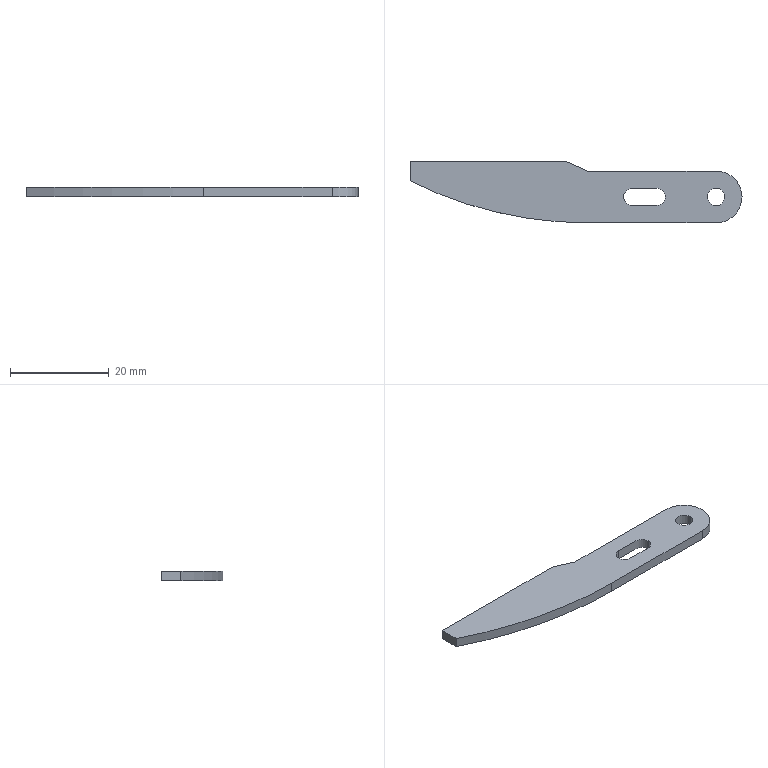Part | SolidWorks | features SMBaseFlange 2, FlatPattern 1, ICE 1, SheetMetal 1 | 1 solid | 17 faces | box 67.25 x 12.5 x 2 mm | volume 1251 mm3 | plane 9 | cylinder 8 | commonest cylinder face diameters 3.5 x5 10.5 x2 160.971 x1
STEP:
#1=CARTESIAN_POINT('',(2.75,0.,-2.));
#2=VERTEX_POINT('',#1);
#3=CARTESIAN_POINT('',(1.,1.75,-2.));
#4=VERTEX_POINT('',#3);
#5=CARTESIAN_POINT('',(1.,0.,-2.));
#6=DIRECTION('',(0.,0.,1.));
#7=DIRECTION('',(1.,0.,0.));
#8=AXIS2_PLACEMENT_3D('',#5,#6,#7);
#9=CIRCLE('',#8,1.75);
#10=EDGE_CURVE('',#2,#4,#9,.T.);
#11=ORIENTED_EDGE('',*,*,#10,.F.);
#12=CARTESIAN_POINT('',(2.75,0.,0.));
#13=VERTEX_POINT('',#12);
#14=CARTESIAN_POINT('',(2.75,0.,-2.));
#15=DIRECTION('',(0.,0.,1.));
#16=VECTOR('',#15,1000.);
#17=LINE('',#14,#16);
#18=EDGE_CURVE('',#2,#13,#17,.T.);
#19=ORIENTED_EDGE('',*,*,#18,.T.);
#20=CARTESIAN_POINT('',(1.,1.75,0.));
#21=VERTEX_POINT('',#20);
#22=CARTESIAN_POINT('',(1.,0.,0.));
#23=DIRECTION('',(0.,0.,1.));
#24=DIRECTION('',(1.,0.,0.));
#25=AXIS2_PLACEMENT_3D('',#22,#23,#24);
#26=CIRCLE('',#25,1.75);
#27=EDGE_CURVE('',#13,#21,#26,.T.);
#28=ORIENTED_EDGE('',*,*,#27,.T.);
#29=CARTESIAN_POINT('',(1.,1.75,-2.));
#30=DIRECTION('',(0.,0.,1.));
#31=VECTOR('',#30,1000.);
#32=LINE('',#29,#31);
#33=EDGE_CURVE('',#4,#21,#32,.T.);
#34=ORIENTED_EDGE('',*,*,#33,.F.);
#35=EDGE_LOOP('',(#11,#19,#28,#34));
#36=FACE_OUTER_BOUND('',#35,.T.);
#37=CARTESIAN_POINT('',(1.,0.,-2.));
#38=DIRECTION('',(0.,0.,1.));
#39=DIRECTION('',(1.,0.,0.));
#40=AXIS2_PLACEMENT_3D('',#37,#38,#39);
#41=CYLINDRICAL_SURFACE('',#40,1.75);
#42=ADVANCED_FACE('',(#36),#41,.F.);
#43=CARTESIAN_POINT('',(11.25,0.,-2.));
#44=VERTEX_POINT('',#43);
#45=CARTESIAN_POINT('',(14.75,0.,-2.));
#46=VERTEX_POINT('',#45);
#47=CARTESIAN_POINT('',(13.,0.,-2.));
#48=DIRECTION('',(0.,0.,1.));
#49=DIRECTION('',(1.,0.,0.));
#50=AXIS2_PLACEMENT_3D('',#47,#48,#49);
#51=CIRCLE('',#50,1.75);
#52=EDGE_CURVE('',#44,#46,#51,.T.);
#53=ORIENTED_EDGE('',*,*,#52,.F.);
#54=CARTESIAN_POINT('',(11.25,0.,0.));
#55=VERTEX_POINT('',#54);
#56=CARTESIAN_POINT('',(11.25,0.,-2.));
#57=DIRECTION('',(0.,0.,1.));
#58=VECTOR('',#57,1000.);
#59=LINE('',#56,#58);
#60=EDGE_CURVE('',#44,#55,#59,.T.);
#61=ORIENTED_EDGE('',*,*,#60,.T.);
#62=CARTESIAN_POINT('',(14.75,0.,0.));
#63=VERTEX_POINT('',#62);
#64=CARTESIAN_POINT('',(13.,0.,0.));
#65=DIRECTION('',(0.,0.,1.));
#66=DIRECTION('',(1.,0.,0.));
#67=AXIS2_PLACEMENT_3D('',#64,#65,#66);
#68=CIRCLE('',#67,1.75);
#69=EDGE_CURVE('',#55,#63,#68,.T.);
#70=ORIENTED_EDGE('',*,*,#69,.T.);
#71=CARTESIAN_POINT('',(14.75,0.,-2.));
#72=DIRECTION('',(0.,0.,1.));
#73=VECTOR('',#72,1000.);
#74=LINE('',#71,#73);
#75=EDGE_CURVE('',#46,#63,#74,.T.);
#76=ORIENTED_EDGE('',*,*,#75,.F.);
#77=EDGE_LOOP('',(#53,#61,#70,#76));
#78=FACE_OUTER_BOUND('',#77,.T.);
#79=CARTESIAN_POINT('',(13.,0.,-2.));
#80=DIRECTION('',(0.,0.,1.));
#81=DIRECTION('',(1.,0.,0.));
#82=AXIS2_PLACEMENT_3D('',#79,#80,#81);
#83=CYLINDRICAL_SURFACE('',#82,1.75);
#84=ADVANCED_FACE('',(#78),#83,.F.);
#85=CARTESIAN_POINT('',(13.,-5.25,-2.));
#86=VERTEX_POINT('',#85);
#87=CARTESIAN_POINT('',(18.25,0.,-2.));
#88=VERTEX_POINT('',#87);
#89=CARTESIAN_POINT('',(13.,0.,-2.));
#90=DIRECTION('',(0.,0.,1.));
#91=DIRECTION('',(1.,0.,0.));
#92=AXIS2_PLACEMENT_3D('',#89,#90,#91);
#93=CIRCLE('',#92,5.25);
#94=EDGE_CURVE('',#86,#88,#93,.T.);
#95=ORIENTED_EDGE('',*,*,#94,.T.);
#96=CARTESIAN_POINT('',(18.25,0.,0.));
#97=VERTEX_POINT('',#96);
#98=CARTESIAN_POINT('',(18.25,0.,-2.));
#99=DIRECTION('',(0.,0.,1.));
#100=VECTOR('',#99,1000.);
#101=LINE('',#98,#100);
#102=EDGE_CURVE('',#88,#97,#101,.T.);
#103=ORIENTED_EDGE('',*,*,#102,.T.);
#104=CARTESIAN_POINT('',(13.,-5.25,0.));
#105=VERTEX_POINT('',#104);
#106=CARTESIAN_POINT('',(13.,0.,0.));
#107=DIRECTION('',(0.,0.,1.));
#108=DIRECTION('',(1.,0.,0.));
#109=AXIS2_PLACEMENT_3D('',#106,#107,#108);
#110=CIRCLE('',#109,5.25);
#111=EDGE_CURVE('',#105,#97,#110,.T.);
#112=ORIENTED_EDGE('',*,*,#111,.F.);
#113=CARTESIAN_POINT('',(13.,-5.25,-2.));
#114=DIRECTION('',(0.,0.,1.));
#115=VECTOR('',#114,1000.);
#116=LINE('',#113,#115);
#117=EDGE_CURVE('',#86,#105,#116,.T.);
#118=ORIENTED_EDGE('',*,*,#117,.F.);
#119=EDGE_LOOP('',(#95,#103,#112,#118));
#120=FACE_OUTER_BOUND('',#119,.T.);
#121=CARTESIAN_POINT('',(13.,0.,-2.));
#122=DIRECTION('',(0.,0.,1.));
#123=DIRECTION('',(1.,0.,0.));
#124=AXIS2_PLACEMENT_3D('',#121,#122,#123);
#125=CYLINDRICAL_SURFACE('',#124,5.25);
#126=ADVANCED_FACE('',(#120),#125,.T.);
#127=ORIENTED_EDGE('',*,*,#102,.F.);
#128=CARTESIAN_POINT('',(13.,5.25,-2.));
#129=VERTEX_POINT('',#128);
#130=CARTESIAN_POINT('',(13.,0.,-2.));
#131=DIRECTION('',(0.,0.,1.));
#132=DIRECTION('',(1.,0.,0.));
#133=AXIS2_PLACEMENT_3D('',#130,#131,#132);
#134=CIRCLE('',#133,5.25);
#135=EDGE_CURVE('',#88,#129,#134,.T.);
#136=ORIENTED_EDGE('',*,*,#135,.T.);
#137=CARTESIAN_POINT('',(13.,5.25,0.));
#138=VERTEX_POINT('',#137);
#139=CARTESIAN_POINT('',(13.,5.25,-2.));
#140=DIRECTION('',(0.,0.,1.));
#141=VECTOR('',#140,1000.);
#142=LINE('',#139,#141);
#143=EDGE_CURVE('',#129,#138,#142,.T.);
#144=ORIENTED_EDGE('',*,*,#143,.T.);
#145=CARTESIAN_POINT('',(13.,0.,0.));
#146=DIRECTION('',(0.,0.,1.));
#147=DIRECTION('',(1.,0.,0.));
#148=AXIS2_PLACEMENT_3D('',#145,#146,#147);
#149=CIRCLE('',#148,5.25);
#150=EDGE_CURVE('',#97,#138,#149,.T.);
#151=ORIENTED_EDGE('',*,*,#150,.F.);
#152=EDGE_LOOP('',(#127,#136,#144,#151));
#153=FACE_OUTER_BOUND('',#152,.T.);
#154=CARTESIAN_POINT('',(13.,0.,-2.));
#155=DIRECTION('',(0.,0.,1.));
#156=DIRECTION('',(1.,0.,0.));
#157=AXIS2_PLACEMENT_3D('',#154,#155,#156);
#158=CYLINDRICAL_SURFACE('',#157,5.25);
#159=ADVANCED_FACE('',(#153),#158,.T.);
#160=CARTESIAN_POINT('',(-13.,-5.25,0.));
#161=VERTEX_POINT('',#160);
#162=CARTESIAN_POINT('',(-13.,-5.25,0.));
#163=DIRECTION('',(1.,0.,0.));
#164=VECTOR('',#163,1000.);
#165=LINE('',#162,#164);
#166=EDGE_CURVE('',#161,#105,#165,.T.);
#167=ORIENTED_EDGE('',*,*,#166,.F.);
#168=CARTESIAN_POINT('',(-13.,-5.25,-2.));
#169=VERTEX_POINT('',#168);
#170=CARTESIAN_POINT('',(-13.,-5.25,-2.));
#171=DIRECTION('',(0.,0.,1.));
#172=VECTOR('',#171,1000.);
#173=LINE('',#170,#172);
#174=EDGE_CURVE('',#169,#161,#173,.T.);
#175=ORIENTED_EDGE('',*,*,#174,.F.);
#176=CARTESIAN_POINT('',(-13.,-5.25,-2.));
#177=DIRECTION('',(1.,0.,0.));
#178=VECTOR('',#177,1000.);
#179=LINE('',#176,#178);
#180=EDGE_CURVE('',#169,#86,#179,.T.);
#181=ORIENTED_EDGE('',*,*,#180,.T.);
#182=ORIENTED_EDGE('',*,*,#117,.T.);
#183=EDGE_LOOP('',(#167,#175,#181,#182));
#184=FACE_OUTER_BOUND('',#183,.T.);
#185=CARTESIAN_POINT('',(-13.,-5.25,-2.));
#186=DIRECTION('',(0.,-1.,0.));
#187=DIRECTION('',(1.,0.,0.));
#188=AXIS2_PLACEMENT_3D('',#185,#186,#187);
#189=PLANE('',#188);
#190=ADVANCED_FACE('',(#184),#189,.T.);
#191=CARTESIAN_POINT('',(-13.,5.25,0.));
#192=VERTEX_POINT('',#191);
#193=CARTESIAN_POINT('',(-13.,5.25,0.));
#194=DIRECTION('',(-1.,0.,0.));
#195=VECTOR('',#194,1000.);
#196=LINE('',#193,#195);
#197=EDGE_CURVE('',#138,#192,#196,.T.);
#198=ORIENTED_EDGE('',*,*,#197,.F.);
#199=ORIENTED_EDGE('',*,*,#143,.F.);
#200=CARTESIAN_POINT('',(-13.,5.25,-2.));
#201=VERTEX_POINT('',#200);
#202=CARTESIAN_POINT('',(-13.,5.25,-2.));
#203=DIRECTION('',(-1.,0.,0.));
#204=VECTOR('',#203,1000.);
#205=LINE('',#202,#204);
#206=EDGE_CURVE('',#129,#201,#205,.T.);
#207=ORIENTED_EDGE('',*,*,#206,.T.);
#208=CARTESIAN_POINT('',(-13.,5.25,-2.));
#209=DIRECTION('',(0.,0.,1.));
#210=VECTOR('',#209,1000.);
#211=LINE('',#208,#210);
#212=EDGE_CURVE('',#201,#192,#211,.T.);
#213=ORIENTED_EDGE('',*,*,#212,.T.);
#214=EDGE_LOOP('',(#198,#199,#207,#213));
#215=FACE_OUTER_BOUND('',#214,.T.);
#216=CARTESIAN_POINT('',(-13.,5.25,-2.));
#217=DIRECTION('',(0.,1.,0.));
#218=DIRECTION('',(-1.,0.,0.));
#219=AXIS2_PLACEMENT_3D('',#216,#217,#218);
#220=PLANE('',#219);
#221=ADVANCED_FACE('',(#215),#220,.T.);
#222=CARTESIAN_POINT('',(-4.,1.75,-2.));
#223=VERTEX_POINT('',#222);
#224=CARTESIAN_POINT('',(-4.,1.75,-2.));
#225=DIRECTION('',(-1.,0.,0.));
#226=VECTOR('',#225,1000.);
#227=LINE('',#224,#226);
#228=EDGE_CURVE('',#4,#223,#227,.T.);
#229=ORIENTED_EDGE('',*,*,#228,.T.);
#230=CARTESIAN_POINT('',(-4.,-1.75,-2.));
#231=VERTEX_POINT('',#230);
#232=CARTESIAN_POINT('',(-4.,0.,-2.));
#233=DIRECTION('',(0.,0.,1.));
#234=DIRECTION('',(1.,0.,0.));
#235=AXIS2_PLACEMENT_3D('',#232,#233,#234);
#236=CIRCLE('',#235,1.75);
#237=EDGE_CURVE('',#223,#231,#236,.T.);
#238=ORIENTED_EDGE('',*,*,#237,.T.);
#239=CARTESIAN_POINT('',(1.,-1.75,-2.));
#240=VERTEX_POINT('',#239);
#241=CARTESIAN_POINT('',(-4.,-1.75,-2.));
#242=DIRECTION('',(1.,0.,0.));
#243=VECTOR('',#242,1000.);
#244=LINE('',#241,#243);
#245=EDGE_CURVE('',#231,#240,#244,.T.);
#246=ORIENTED_EDGE('',*,*,#245,.T.);
#247=CARTESIAN_POINT('',(1.,0.,-2.));
#248=DIRECTION('',(0.,0.,1.));
#249=DIRECTION('',(1.,0.,0.));
#250=AXIS2_PLACEMENT_3D('',#247,#248,#249);
#251=CIRCLE('',#250,1.75);
#252=EDGE_CURVE('',#240,#2,#251,.T.);
#253=ORIENTED_EDGE('',*,*,#252,.T.);
#254=ORIENTED_EDGE('',*,*,#10,.T.);
#255=EDGE_LOOP('',(#229,#238,#246,#253,#254));
#256=FACE_BOUND('',#255,.T.);
#257=CARTESIAN_POINT('',(13.,0.,-2.));
#258=DIRECTION('',(0.,0.,1.));
#259=DIRECTION('',(1.,0.,0.));
#260=AXIS2_PLACEMENT_3D('',#257,#258,#259);
#261=CIRCLE('',#260,1.75);
#262=EDGE_CURVE('',#46,#44,#261,.T.);
#263=ORIENTED_EDGE('',*,*,#262,.T.);
#264=ORIENTED_EDGE('',*,*,#52,.T.);
#265=EDGE_LOOP('',(#263,#264));
#266=FACE_BOUND('',#265,.T.);
#267=ORIENTED_EDGE('',*,*,#94,.F.);
#268=ORIENTED_EDGE('',*,*,#180,.F.);
#269=CARTESIAN_POINT('',(-49.,3.25,-2.));
#270=VERTEX_POINT('',#269);
#271=CARTESIAN_POINT('',(-13.,75.235,-2.));
#272=DIRECTION('',(0.,0.,1.));
#273=DIRECTION('',(1.,0.,0.));
#274=AXIS2_PLACEMENT_3D('',#271,#272,#273);
#275=CIRCLE('',#274,80.485);
#276=EDGE_CURVE('',#270,#169,#275,.T.);
#277=ORIENTED_EDGE('',*,*,#276,.F.);
#278=CARTESIAN_POINT('',(-49.,7.25,-2.));
#279=VERTEX_POINT('',#278);
#280=CARTESIAN_POINT('',(-49.,7.25,-2.));
#281=DIRECTION('',(0.,-1.,0.));
#282=VECTOR('',#281,1000.);
#283=LINE('',#280,#282);
#284=EDGE_CURVE('',#279,#270,#283,.T.);
#285=ORIENTED_EDGE('',*,*,#284,.F.);
#286=CARTESIAN_POINT('',(-17.5,7.25,-2.));
#287=VERTEX_POINT('',#286);
#288=CARTESIAN_POINT('',(-17.5,7.25,-2.));
#289=DIRECTION('',(-1.,0.,0.));
#290=VECTOR('',#289,1000.);
#291=LINE('',#288,#290);
#292=EDGE_CURVE('',#287,#279,#291,.T.);
#293=ORIENTED_EDGE('',*,*,#292,.F.);
#294=CARTESIAN_POINT('',(-13.,5.25,-2.));
#295=DIRECTION('',(-0.9138,0.4061,0.));
#296=VECTOR('',#295,1000.);
#297=LINE('',#294,#296);
#298=EDGE_CURVE('',#201,#287,#297,.T.);
#299=ORIENTED_EDGE('',*,*,#298,.F.);
#300=ORIENTED_EDGE('',*,*,#206,.F.);
#301=ORIENTED_EDGE('',*,*,#135,.F.);
#302=EDGE_LOOP('',(#267,#268,#277,#285,#293,#299,#300,#301));
#303=FACE_OUTER_BOUND('',#302,.T.);
#304=CARTESIAN_POINT('',(13.,0.,-2.));
#305=DIRECTION('',(0.,0.,1.));
#306=DIRECTION('',(1.,0.,0.));
#307=AXIS2_PLACEMENT_3D('',#304,#305,#306);
#308=PLANE('',#307);
#309=ADVANCED_FACE('',(#256,#266,#303),#308,.F.);
#310=CARTESIAN_POINT('',(-4.,1.75,0.));
#311=VERTEX_POINT('',#310);
#312=CARTESIAN_POINT('',(-4.,-1.75,0.));
#313=VERTEX_POINT('',#312);
#314=CARTESIAN_POINT('',(-4.,0.,0.));
#315=DIRECTION('',(0.,0.,1.));
#316=DIRECTION('',(1.,0.,0.));
#317=AXIS2_PLACEMENT_3D('',#314,#315,#316);
#318=CIRCLE('',#317,1.75);
#319=EDGE_CURVE('',#311,#313,#318,.T.);
#320=ORIENTED_EDGE('',*,*,#319,.F.);
#321=CARTESIAN_POINT('',(-4.,1.75,0.));
#322=DIRECTION('',(-1.,0.,0.));
#323=VECTOR('',#322,1000.);
#324=LINE('',#321,#323);
#325=EDGE_CURVE('',#21,#311,#324,.T.);
#326=ORIENTED_EDGE('',*,*,#325,.F.);
#327=ORIENTED_EDGE('',*,*,#27,.F.);
#328=CARTESIAN_POINT('',(1.,-1.75,0.));
#329=VERTEX_POINT('',#328);
#330=CARTESIAN_POINT('',(1.,0.,0.));
#331=DIRECTION('',(0.,0.,1.));
#332=DIRECTION('',(1.,0.,0.));
#333=AXIS2_PLACEMENT_3D('',#330,#331,#332);
#334=CIRCLE('',#333,1.75);
#335=EDGE_CURVE('',#329,#13,#334,.T.);
#336=ORIENTED_EDGE('',*,*,#335,.F.);
#337=CARTESIAN_POINT('',(-4.,-1.75,0.));
#338=DIRECTION('',(1.,0.,0.));
#339=VECTOR('',#338,1000.);
#340=LINE('',#337,#339);
#341=EDGE_CURVE('',#313,#329,#340,.T.);
#342=ORIENTED_EDGE('',*,*,#341,.F.);
#343=EDGE_LOOP('',(#320,#326,#327,#336,#342));
#344=FACE_BOUND('',#343,.T.);
#345=CARTESIAN_POINT('',(13.,0.,0.));
#346=DIRECTION('',(0.,0.,1.));
#347=DIRECTION('',(1.,0.,0.));
#348=AXIS2_PLACEMENT_3D('',#345,#346,#347);
#349=CIRCLE('',#348,1.75);
#350=EDGE_CURVE('',#63,#55,#349,.T.);
#351=ORIENTED_EDGE('',*,*,#350,.F.);
#352=ORIENTED_EDGE('',*,*,#69,.F.);
#353=EDGE_LOOP('',(#351,#352));
#354=FACE_BOUND('',#353,.T.);
#355=ORIENTED_EDGE('',*,*,#111,.T.);
#356=ORIENTED_EDGE('',*,*,#150,.T.);
#357=ORIENTED_EDGE('',*,*,#197,.T.);
#358=CARTESIAN_POINT('',(-17.5,7.25,0.));
#359=VERTEX_POINT('',#358);
#360=CARTESIAN_POINT('',(-13.,5.25,0.));
#361=DIRECTION('',(-0.9138,0.4061,0.));
#362=VECTOR('',#361,1000.);
#363=LINE('',#360,#362);
#364=EDGE_CURVE('',#192,#359,#363,.T.);
#365=ORIENTED_EDGE('',*,*,#364,.T.);
#366=CARTESIAN_POINT('',(-49.,7.25,0.));
#367=VERTEX_POINT('',#366);
#368=CARTESIAN_POINT('',(-17.5,7.25,0.));
#369=DIRECTION('',(-1.,0.,0.));
#370=VECTOR('',#369,1000.);
#371=LINE('',#368,#370);
#372=EDGE_CURVE('',#359,#367,#371,.T.);
#373=ORIENTED_EDGE('',*,*,#372,.T.);
#374=CARTESIAN_POINT('',(-49.,3.25,0.));
#375=VERTEX_POINT('',#374);
#376=CARTESIAN_POINT('',(-49.,7.25,0.));
#377=DIRECTION('',(0.,-1.,0.));
#378=VECTOR('',#377,1000.);
#379=LINE('',#376,#378);
#380=EDGE_CURVE('',#367,#375,#379,.T.);
#381=ORIENTED_EDGE('',*,*,#380,.T.);
#382=CARTESIAN_POINT('',(-13.,75.235,0.));
#383=DIRECTION('',(0.,0.,1.));
#384=DIRECTION('',(1.,0.,0.));
#385=AXIS2_PLACEMENT_3D('',#382,#383,#384);
#386=CIRCLE('',#385,80.485);
#387=EDGE_CURVE('',#375,#161,#386,.T.);
#388=ORIENTED_EDGE('',*,*,#387,.T.);
#389=ORIENTED_EDGE('',*,*,#166,.T.);
#390=EDGE_LOOP('',(#355,#356,#357,#365,#373,#381,#388,#389));
#391=FACE_OUTER_BOUND('',#390,.T.);
#392=CARTESIAN_POINT('',(13.,0.,0.));
#393=DIRECTION('',(0.,0.,1.));
#394=DIRECTION('',(1.,0.,0.));
#395=AXIS2_PLACEMENT_3D('',#392,#393,#394);
#396=PLANE('',#395);
#397=ADVANCED_FACE('',(#344,#354,#391),#396,.T.);
#398=ORIENTED_EDGE('',*,*,#60,.F.);
#399=ORIENTED_EDGE('',*,*,#262,.F.);
#400=ORIENTED_EDGE('',*,*,#75,.T.);
#401=ORIENTED_EDGE('',*,*,#350,.T.);
#402=EDGE_LOOP('',(#398,#399,#400,#401));
#403=FACE_OUTER_BOUND('',#402,.T.);
#404=CARTESIAN_POINT('',(13.,0.,-2.));
#405=DIRECTION('',(0.,0.,1.));
#406=DIRECTION('',(1.,0.,0.));
#407=AXIS2_PLACEMENT_3D('',#404,#405,#406);
#408=CYLINDRICAL_SURFACE('',#407,1.75);
#409=ADVANCED_FACE('',(#403),#408,.F.);
#410=ORIENTED_EDGE('',*,*,#387,.F.);
#411=CARTESIAN_POINT('',(-49.,3.25,-2.));
#412=DIRECTION('',(0.,0.,1.));
#413=VECTOR('',#412,1000.);
#414=LINE('',#411,#413);
#415=EDGE_CURVE('',#270,#375,#414,.T.);
#416=ORIENTED_EDGE('',*,*,#415,.F.);
#417=ORIENTED_EDGE('',*,*,#276,.T.);
#418=ORIENTED_EDGE('',*,*,#174,.T.);
#419=EDGE_LOOP('',(#410,#416,#417,#418));
#420=FACE_OUTER_BOUND('',#419,.T.);
#421=CARTESIAN_POINT('',(-13.,75.235,-2.));
#422=DIRECTION('',(0.,0.,1.));
#423=DIRECTION('',(1.,0.,0.));
#424=AXIS2_PLACEMENT_3D('',#421,#422,#423);
#425=CYLINDRICAL_SURFACE('',#424,80.485);
#426=ADVANCED_FACE('',(#420),#425,.T.);
#427=ORIENTED_EDGE('',*,*,#380,.F.);
#428=CARTESIAN_POINT('',(-49.,7.25,-2.));
#429=DIRECTION('',(0.,0.,1.));
#430=VECTOR('',#429,1000.);
#431=LINE('',#428,#430);
#432=EDGE_CURVE('',#279,#367,#431,.T.);
#433=ORIENTED_EDGE('',*,*,#432,.F.);
#434=ORIENTED_EDGE('',*,*,#284,.T.);
#435=ORIENTED_EDGE('',*,*,#415,.T.);
#436=EDGE_LOOP('',(#427,#433,#434,#435));
#437=FACE_OUTER_BOUND('',#436,.T.);
#438=CARTESIAN_POINT('',(-49.,7.25,-2.));
#439=DIRECTION('',(-1.,0.,0.));
#440=DIRECTION('',(0.,0.,1.));
#441=AXIS2_PLACEMENT_3D('',#438,#439,#440);
#442=PLANE('',#441);
#443=ADVANCED_FACE('',(#437),#442,.T.);
#444=ORIENTED_EDGE('',*,*,#372,.F.);
#445=CARTESIAN_POINT('',(-17.5,7.25,-2.));
#446=DIRECTION('',(0.,0.,1.));
#447=VECTOR('',#446,1000.);
#448=LINE('',#445,#447);
#449=EDGE_CURVE('',#287,#359,#448,.T.);
#450=ORIENTED_EDGE('',*,*,#449,.F.);
#451=ORIENTED_EDGE('',*,*,#292,.T.);
#452=ORIENTED_EDGE('',*,*,#432,.T.);
#453=EDGE_LOOP('',(#444,#450,#451,#452));
#454=FACE_OUTER_BOUND('',#453,.T.);
#455=CARTESIAN_POINT('',(-17.5,7.25,-2.));
#456=DIRECTION('',(0.,1.,0.));
#457=DIRECTION('',(-1.,0.,0.));
#458=AXIS2_PLACEMENT_3D('',#455,#456,#457);
#459=PLANE('',#458);
#460=ADVANCED_FACE('',(#454),#459,.T.);
#461=ORIENTED_EDGE('',*,*,#364,.F.);
#462=ORIENTED_EDGE('',*,*,#212,.F.);
#463=ORIENTED_EDGE('',*,*,#298,.T.);
#464=ORIENTED_EDGE('',*,*,#449,.T.);
#465=EDGE_LOOP('',(#461,#462,#463,#464));
#466=FACE_OUTER_BOUND('',#465,.T.);
#467=CARTESIAN_POINT('',(-13.,5.25,-2.));
#468=DIRECTION('',(0.4061,0.9138,0.));
#469=DIRECTION('',(-0.9138,0.4061,0.));
#470=AXIS2_PLACEMENT_3D('',#467,#468,#469);
#471=PLANE('',#470);
#472=ADVANCED_FACE('',(#466),#471,.T.);
#473=ORIENTED_EDGE('',*,*,#319,.T.);
#474=CARTESIAN_POINT('',(-4.,-1.75,-2.));
#475=DIRECTION('',(0.,0.,1.));
#476=VECTOR('',#475,1000.);
#477=LINE('',#474,#476);
#478=EDGE_CURVE('',#231,#313,#477,.T.);
#479=ORIENTED_EDGE('',*,*,#478,.F.);
#480=ORIENTED_EDGE('',*,*,#237,.F.);
#481=CARTESIAN_POINT('',(-4.,1.75,-2.));
#482=DIRECTION('',(0.,0.,1.));
#483=VECTOR('',#482,1000.);
#484=LINE('',#481,#483);
#485=EDGE_CURVE('',#223,#311,#484,.T.);
#486=ORIENTED_EDGE('',*,*,#485,.T.);
#487=EDGE_LOOP('',(#473,#479,#480,#486));
#488=FACE_OUTER_BOUND('',#487,.T.);
#489=CARTESIAN_POINT('',(-4.,0.,-2.));
#490=DIRECTION('',(0.,0.,1.));
#491=DIRECTION('',(1.,0.,0.));
#492=AXIS2_PLACEMENT_3D('',#489,#490,#491);
#493=CYLINDRICAL_SURFACE('',#492,1.75);
#494=ADVANCED_FACE('',(#488),#493,.F.);
#495=ORIENTED_EDGE('',*,*,#325,.T.);
#496=ORIENTED_EDGE('',*,*,#485,.F.);
#497=ORIENTED_EDGE('',*,*,#228,.F.);
#498=ORIENTED_EDGE('',*,*,#33,.T.);
#499=EDGE_LOOP('',(#495,#496,#497,#498));
#500=FACE_OUTER_BOUND('',#499,.T.);
#501=CARTESIAN_POINT('',(-4.,1.75,-2.));
#502=DIRECTION('',(0.,1.,0.));
#503=DIRECTION('',(0.,0.,1.));
#504=AXIS2_PLACEMENT_3D('',#501,#502,#503);
#505=PLANE('',#504);
#506=ADVANCED_FACE('',(#500),#505,.F.);
#507=ORIENTED_EDGE('',*,*,#18,.F.);
#508=ORIENTED_EDGE('',*,*,#252,.F.);
#509=CARTESIAN_POINT('',(1.,-1.75,-2.));
#510=DIRECTION('',(0.,0.,1.));
#511=VECTOR('',#510,1000.);
#512=LINE('',#509,#511);
#513=EDGE_CURVE('',#240,#329,#512,.T.);
#514=ORIENTED_EDGE('',*,*,#513,.T.);
#515=ORIENTED_EDGE('',*,*,#335,.T.);
#516=EDGE_LOOP('',(#507,#508,#514,#515));
#517=FACE_OUTER_BOUND('',#516,.T.);
#518=CARTESIAN_POINT('',(1.,0.,-2.));
#519=DIRECTION('',(0.,0.,1.));
#520=DIRECTION('',(1.,0.,0.));
#521=AXIS2_PLACEMENT_3D('',#518,#519,#520);
#522=CYLINDRICAL_SURFACE('',#521,1.75);
#523=ADVANCED_FACE('',(#517),#522,.F.);
#524=ORIENTED_EDGE('',*,*,#341,.T.);
#525=ORIENTED_EDGE('',*,*,#513,.F.);
#526=ORIENTED_EDGE('',*,*,#245,.F.);
#527=ORIENTED_EDGE('',*,*,#478,.T.);
#528=EDGE_LOOP('',(#524,#525,#526,#527));
#529=FACE_OUTER_BOUND('',#528,.T.);
#530=CARTESIAN_POINT('',(-4.,-1.75,-2.));
#531=DIRECTION('',(0.,-1.,0.));
#532=DIRECTION('',(0.,0.,-1.));
#533=AXIS2_PLACEMENT_3D('',#530,#531,#532);
#534=PLANE('',#533);
#535=ADVANCED_FACE('',(#529),#534,.F.);
#536=CLOSED_SHELL('',(#42,#84,#126,#159,#190,#221,#309,#397,#409,#426,#443,#460,#472,#494,#506,#523,#535));
#537=MANIFOLD_SOLID_BREP('',#536);
#538=CARTESIAN_POINT('',(0.,0.,0.));
#539=DIRECTION('',(0.,0.,1.));
#540=DIRECTION('',(1.,0.,0.));
#541=AXIS2_PLACEMENT_3D('',#538,#539,#540);
#542=(LENGTH_UNIT()NAMED_UNIT(*)SI_UNIT(.MILLI.,.METRE.));
#543=UNCERTAINTY_MEASURE_WITH_UNIT(LENGTH_MEASURE(0.00001),#542,'','');
#544=(NAMED_UNIT(*)PLANE_ANGLE_UNIT()SI_UNIT($,.RADIAN.));
#545=(NAMED_UNIT(*)SI_UNIT($,.STERADIAN.)SOLID_ANGLE_UNIT());
#546=(GEOMETRIC_REPRESENTATION_CONTEXT(3)GLOBAL_UNCERTAINTY_ASSIGNED_CONTEXT((#543))GLOBAL_UNIT_ASSIGNED_CONTEXT((#542,#544,#545))REPRESENTATION_CONTEXT('',''));
#547=ADVANCED_BREP_SHAPE_REPRESENTATION('',(#537,#541),#546);